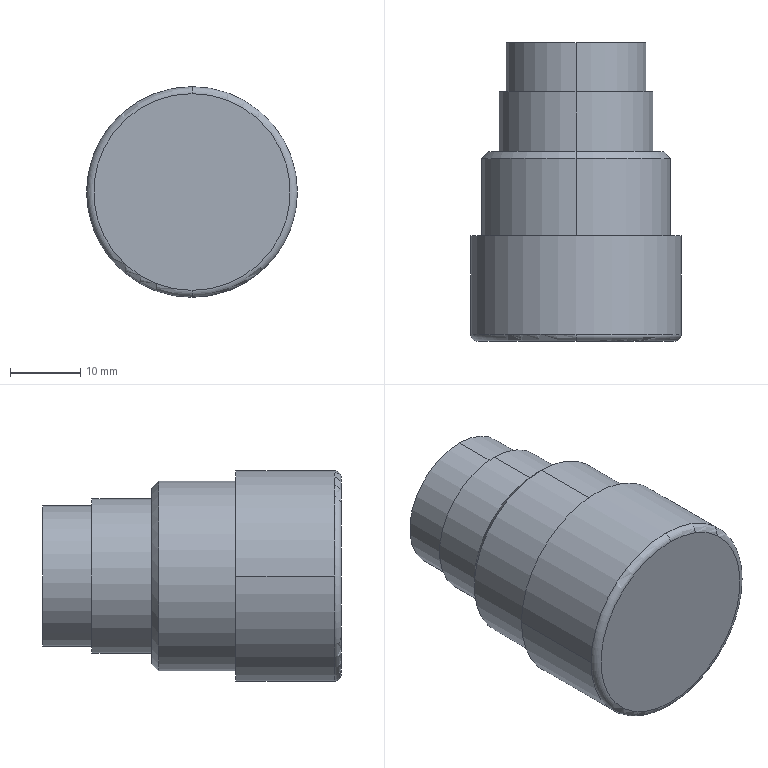Part | SolidWorks | features ICE 2, BaseBody 1, Fillet 1 | 1 solid | 20 faces | box 30 x 42.5 x 30 mm | volume 22079 mm3 | cylinder 10 | plane 6 | torus 2 | cone 2 | commonest cylinder face diameters 18 x2 20 x2 22 x2 27 x2 30 x2
STEP:
#1=CARTESIAN_POINT('',(0.,4.,-14.));
#2=VERTEX_POINT('',#1);
#3=CARTESIAN_POINT('',(0.,4.,14.));
#4=VERTEX_POINT('',#3);
#5=CARTESIAN_POINT('',(0.,4.,0.));
#6=DIRECTION('',(0.,-1.,0.));
#7=DIRECTION('',(0.,0.,1.));
#8=AXIS2_PLACEMENT_3D('',#5,#6,#7);
#9=CIRCLE('',#8,14.);
#10=EDGE_CURVE('',#2,#4,#9,.T.);
#11=ORIENTED_EDGE('',*,*,#10,.F.);
#12=CARTESIAN_POINT('',(0.,5.,-15.));
#13=VERTEX_POINT('',#12);
#14=CARTESIAN_POINT('',(0.,5.,-14.));
#15=DIRECTION('',(1.,0.,0.));
#16=DIRECTION('',(0.,0.,-1.));
#17=AXIS2_PLACEMENT_3D('',#14,#15,#16);
#18=CIRCLE('',#17,1.);
#19=EDGE_CURVE('',#2,#13,#18,.T.);
#20=ORIENTED_EDGE('',*,*,#19,.T.);
#21=CARTESIAN_POINT('',(15.,5.,0.));
#22=VERTEX_POINT('',#21);
#23=CARTESIAN_POINT('',(0.,5.,0.));
#24=DIRECTION('',(0.,1.,0.));
#25=DIRECTION('',(0.,0.,1.));
#26=AXIS2_PLACEMENT_3D('',#23,#24,#25);
#27=CIRCLE('',#26,15.);
#28=EDGE_CURVE('',#22,#13,#27,.T.);
#29=ORIENTED_EDGE('',*,*,#28,.F.);
#30=CARTESIAN_POINT('',(0.,5.,15.));
#31=VERTEX_POINT('',#30);
#32=CARTESIAN_POINT('',(0.,5.,0.));
#33=DIRECTION('',(0.,1.,0.));
#34=DIRECTION('',(0.,0.,1.));
#35=AXIS2_PLACEMENT_3D('',#32,#33,#34);
#36=CIRCLE('',#35,15.);
#37=EDGE_CURVE('',#31,#22,#36,.T.);
#38=ORIENTED_EDGE('',*,*,#37,.F.);
#39=CARTESIAN_POINT('',(0.,5.,14.));
#40=DIRECTION('',(-1.,0.,0.));
#41=DIRECTION('',(0.,0.,1.));
#42=AXIS2_PLACEMENT_3D('',#39,#40,#41);
#43=CIRCLE('',#42,1.);
#44=EDGE_CURVE('',#4,#31,#43,.T.);
#45=ORIENTED_EDGE('',*,*,#44,.F.);
#46=EDGE_LOOP('',(#11,#20,#29,#38,#45));
#47=FACE_OUTER_BOUND('',#46,.T.);
#48=CARTESIAN_POINT('',(0.,5.,0.));
#49=DIRECTION('',(0.,1.,0.));
#50=DIRECTION('',(0.,0.,1.));
#51=AXIS2_PLACEMENT_3D('',#48,#49,#50);
#52=TOROIDAL_SURFACE('',#51,14.,1.);
#53=ADVANCED_FACE('',(#47),#52,.T.);
#54=ORIENTED_EDGE('',*,*,#28,.T.);
#55=CARTESIAN_POINT('',(-15.,5.,0.));
#56=VERTEX_POINT('',#55);
#57=CARTESIAN_POINT('',(0.,5.,0.));
#58=DIRECTION('',(0.,1.,0.));
#59=DIRECTION('',(0.,0.,1.));
#60=AXIS2_PLACEMENT_3D('',#57,#58,#59);
#61=CIRCLE('',#60,15.);
#62=EDGE_CURVE('',#13,#56,#61,.T.);
#63=ORIENTED_EDGE('',*,*,#62,.T.);
#64=CARTESIAN_POINT('',(-15.,19.,0.));
#65=VERTEX_POINT('',#64);
#66=CARTESIAN_POINT('',(-15.,6.,0.));
#67=DIRECTION('',(0.,1.,0.));
#68=VECTOR('',#67,1000.);
#69=LINE('',#66,#68);
#70=EDGE_CURVE('',#56,#65,#69,.T.);
#71=ORIENTED_EDGE('',*,*,#70,.T.);
#72=CARTESIAN_POINT('',(15.,19.,0.));
#73=VERTEX_POINT('',#72);
#74=CARTESIAN_POINT('',(0.,19.,0.));
#75=DIRECTION('',(0.,1.,0.));
#76=DIRECTION('',(1.,0.,0.));
#77=AXIS2_PLACEMENT_3D('',#74,#75,#76);
#78=CIRCLE('',#77,15.);
#79=EDGE_CURVE('',#73,#65,#78,.T.);
#80=ORIENTED_EDGE('',*,*,#79,.F.);
#81=CARTESIAN_POINT('',(15.,6.,0.));
#82=DIRECTION('',(0.,1.,0.));
#83=VECTOR('',#82,1000.);
#84=LINE('',#81,#83);
#85=EDGE_CURVE('',#22,#73,#84,.T.);
#86=ORIENTED_EDGE('',*,*,#85,.F.);
#87=EDGE_LOOP('',(#54,#63,#71,#80,#86));
#88=FACE_OUTER_BOUND('',#87,.T.);
#89=CARTESIAN_POINT('',(0.,6.,0.));
#90=DIRECTION('',(0.,1.,0.));
#91=DIRECTION('',(1.,0.,0.));
#92=AXIS2_PLACEMENT_3D('',#89,#90,#91);
#93=CYLINDRICAL_SURFACE('',#92,15.);
#94=ADVANCED_FACE('',(#88),#93,.T.);
#95=CARTESIAN_POINT('',(9.,43.5,0.));
#96=VERTEX_POINT('',#95);
#97=CARTESIAN_POINT('',(-9.,43.5,0.));
#98=VERTEX_POINT('',#97);
#99=CARTESIAN_POINT('',(0.,43.5,0.));
#100=DIRECTION('',(0.,1.,0.));
#101=DIRECTION('',(1.,0.,0.));
#102=AXIS2_PLACEMENT_3D('',#99,#100,#101);
#103=CIRCLE('',#102,9.);
#104=EDGE_CURVE('',#96,#98,#103,.T.);
#105=ORIENTED_EDGE('',*,*,#104,.T.);
#106=CARTESIAN_POINT('',(0.,43.5,0.));
#107=DIRECTION('',(0.,1.,0.));
#108=DIRECTION('',(-1.,0.,0.));
#109=AXIS2_PLACEMENT_3D('',#106,#107,#108);
#110=CIRCLE('',#109,9.);
#111=EDGE_CURVE('',#98,#96,#110,.T.);
#112=ORIENTED_EDGE('',*,*,#111,.T.);
#113=EDGE_LOOP('',(#105,#112));
#114=FACE_OUTER_BOUND('',#113,.T.);
#115=CARTESIAN_POINT('',(0.,43.5,0.));
#116=DIRECTION('',(0.,1.,0.));
#117=DIRECTION('',(-1.,0.,0.));
#118=AXIS2_PLACEMENT_3D('',#115,#116,#117);
#119=PLANE('',#118);
#120=ADVANCED_FACE('',(#114),#119,.T.);
#121=CARTESIAN_POINT('',(-9.,46.5,0.));
#122=VERTEX_POINT('',#121);
#123=CARTESIAN_POINT('',(-9.,46.5,0.));
#124=DIRECTION('',(0.,-1.,0.));
#125=VECTOR('',#124,1000.);
#126=LINE('',#123,#125);
#127=EDGE_CURVE('',#122,#98,#126,.T.);
#128=ORIENTED_EDGE('',*,*,#127,.T.);
#129=ORIENTED_EDGE('',*,*,#104,.F.);
#130=CARTESIAN_POINT('',(9.,46.5,0.));
#131=VERTEX_POINT('',#130);
#132=CARTESIAN_POINT('',(9.,46.5,0.));
#133=DIRECTION('',(0.,-1.,0.));
#134=VECTOR('',#133,1000.);
#135=LINE('',#132,#134);
#136=EDGE_CURVE('',#131,#96,#135,.T.);
#137=ORIENTED_EDGE('',*,*,#136,.F.);
#138=CARTESIAN_POINT('',(0.,46.5,0.));
#139=DIRECTION('',(0.,1.,0.));
#140=DIRECTION('',(1.,0.,0.));
#141=AXIS2_PLACEMENT_3D('',#138,#139,#140);
#142=CIRCLE('',#141,9.);
#143=EDGE_CURVE('',#131,#122,#142,.T.);
#144=ORIENTED_EDGE('',*,*,#143,.T.);
#145=EDGE_LOOP('',(#128,#129,#137,#144));
#146=FACE_OUTER_BOUND('',#145,.T.);
#147=CARTESIAN_POINT('',(0.,46.5,0.));
#148=DIRECTION('',(0.,1.,0.));
#149=DIRECTION('',(-1.,0.,0.));
#150=AXIS2_PLACEMENT_3D('',#147,#148,#149);
#151=CYLINDRICAL_SURFACE('',#150,9.);
#152=ADVANCED_FACE('',(#146),#151,.F.);
#153=ORIENTED_EDGE('',*,*,#136,.T.);
#154=ORIENTED_EDGE('',*,*,#111,.F.);
#155=ORIENTED_EDGE('',*,*,#127,.F.);
#156=CARTESIAN_POINT('',(0.,46.5,0.));
#157=DIRECTION('',(0.,1.,0.));
#158=DIRECTION('',(-1.,0.,0.));
#159=AXIS2_PLACEMENT_3D('',#156,#157,#158);
#160=CIRCLE('',#159,9.);
#161=EDGE_CURVE('',#122,#131,#160,.T.);
#162=ORIENTED_EDGE('',*,*,#161,.T.);
#163=EDGE_LOOP('',(#153,#154,#155,#162));
#164=FACE_OUTER_BOUND('',#163,.T.);
#165=CARTESIAN_POINT('',(0.,46.5,0.));
#166=DIRECTION('',(0.,1.,0.));
#167=DIRECTION('',(-1.,0.,0.));
#168=AXIS2_PLACEMENT_3D('',#165,#166,#167);
#169=CYLINDRICAL_SURFACE('',#168,9.);
#170=ADVANCED_FACE('',(#164),#169,.F.);
#171=ORIENTED_EDGE('',*,*,#143,.F.);
#172=ORIENTED_EDGE('',*,*,#161,.F.);
#173=EDGE_LOOP('',(#171,#172));
#174=FACE_BOUND('',#173,.T.);
#175=CARTESIAN_POINT('',(0.,46.5,10.));
#176=VERTEX_POINT('',#175);
#177=CARTESIAN_POINT('',(0.,46.5,-10.));
#178=VERTEX_POINT('',#177);
#179=CARTESIAN_POINT('',(0.,46.5,0.));
#180=DIRECTION('',(0.,1.,0.));
#181=DIRECTION('',(0.,0.,1.));
#182=AXIS2_PLACEMENT_3D('',#179,#180,#181);
#183=CIRCLE('',#182,10.);
#184=EDGE_CURVE('',#176,#178,#183,.T.);
#185=ORIENTED_EDGE('',*,*,#184,.T.);
#186=CARTESIAN_POINT('',(0.,46.5,0.));
#187=DIRECTION('',(0.,1.,0.));
#188=DIRECTION('',(0.,0.,-1.));
#189=AXIS2_PLACEMENT_3D('',#186,#187,#188);
#190=CIRCLE('',#189,10.);
#191=EDGE_CURVE('',#178,#176,#190,.T.);
#192=ORIENTED_EDGE('',*,*,#191,.T.);
#193=EDGE_LOOP('',(#185,#192));
#194=FACE_OUTER_BOUND('',#193,.T.);
#195=CARTESIAN_POINT('',(0.,46.5,0.));
#196=DIRECTION('',(0.,1.,0.));
#197=DIRECTION('',(0.,0.,-1.));
#198=AXIS2_PLACEMENT_3D('',#195,#196,#197);
#199=PLANE('',#198);
#200=ADVANCED_FACE('',(#174,#194),#199,.T.);
#201=CARTESIAN_POINT('',(0.,39.5,-10.));
#202=VERTEX_POINT('',#201);
#203=CARTESIAN_POINT('',(0.,39.5,-10.));
#204=DIRECTION('',(0.,1.,0.));
#205=VECTOR('',#204,1000.);
#206=LINE('',#203,#205);
#207=EDGE_CURVE('',#202,#178,#206,.T.);
#208=ORIENTED_EDGE('',*,*,#207,.T.);
#209=ORIENTED_EDGE('',*,*,#184,.F.);
#210=CARTESIAN_POINT('',(0.,39.5,10.));
#211=VERTEX_POINT('',#210);
#212=CARTESIAN_POINT('',(0.,39.5,10.));
#213=DIRECTION('',(0.,1.,0.));
#214=VECTOR('',#213,1000.);
#215=LINE('',#212,#214);
#216=EDGE_CURVE('',#211,#176,#215,.T.);
#217=ORIENTED_EDGE('',*,*,#216,.F.);
#218=CARTESIAN_POINT('',(0.,39.5,0.));
#219=DIRECTION('',(0.,1.,0.));
#220=DIRECTION('',(0.,0.,1.));
#221=AXIS2_PLACEMENT_3D('',#218,#219,#220);
#222=CIRCLE('',#221,10.);
#223=EDGE_CURVE('',#211,#202,#222,.T.);
#224=ORIENTED_EDGE('',*,*,#223,.T.);
#225=EDGE_LOOP('',(#208,#209,#217,#224));
#226=FACE_OUTER_BOUND('',#225,.T.);
#227=CARTESIAN_POINT('',(0.,39.5,0.));
#228=DIRECTION('',(0.,1.,0.));
#229=DIRECTION('',(0.,0.,-1.));
#230=AXIS2_PLACEMENT_3D('',#227,#228,#229);
#231=CYLINDRICAL_SURFACE('',#230,10.);
#232=ADVANCED_FACE('',(#226),#231,.T.);
#233=ORIENTED_EDGE('',*,*,#216,.T.);
#234=ORIENTED_EDGE('',*,*,#191,.F.);
#235=ORIENTED_EDGE('',*,*,#207,.F.);
#236=CARTESIAN_POINT('',(0.,39.5,0.));
#237=DIRECTION('',(0.,1.,0.));
#238=DIRECTION('',(0.,0.,-1.));
#239=AXIS2_PLACEMENT_3D('',#236,#237,#238);
#240=CIRCLE('',#239,10.);
#241=EDGE_CURVE('',#202,#211,#240,.T.);
#242=ORIENTED_EDGE('',*,*,#241,.T.);
#243=EDGE_LOOP('',(#233,#234,#235,#242));
#244=FACE_OUTER_BOUND('',#243,.T.);
#245=CARTESIAN_POINT('',(0.,39.5,0.));
#246=DIRECTION('',(0.,1.,0.));
#247=DIRECTION('',(0.,0.,-1.));
#248=AXIS2_PLACEMENT_3D('',#245,#246,#247);
#249=CYLINDRICAL_SURFACE('',#248,10.);
#250=ADVANCED_FACE('',(#244),#249,.T.);
#251=ORIENTED_EDGE('',*,*,#223,.F.);
#252=ORIENTED_EDGE('',*,*,#241,.F.);
#253=EDGE_LOOP('',(#251,#252));
#254=FACE_BOUND('',#253,.T.);
#255=CARTESIAN_POINT('',(0.,39.5,11.));
#256=VERTEX_POINT('',#255);
#257=CARTESIAN_POINT('',(0.,39.5,-11.));
#258=VERTEX_POINT('',#257);
#259=CARTESIAN_POINT('',(0.,39.5,0.));
#260=DIRECTION('',(0.,1.,0.));
#261=DIRECTION('',(0.,0.,1.));
#262=AXIS2_PLACEMENT_3D('',#259,#260,#261);
#263=CIRCLE('',#262,11.);
#264=EDGE_CURVE('',#256,#258,#263,.T.);
#265=ORIENTED_EDGE('',*,*,#264,.T.);
#266=CARTESIAN_POINT('',(0.,39.5,0.));
#267=DIRECTION('',(0.,1.,0.));
#268=DIRECTION('',(0.,0.,-1.));
#269=AXIS2_PLACEMENT_3D('',#266,#267,#268);
#270=CIRCLE('',#269,11.);
#271=EDGE_CURVE('',#258,#256,#270,.T.);
#272=ORIENTED_EDGE('',*,*,#271,.T.);
#273=EDGE_LOOP('',(#265,#272));
#274=FACE_OUTER_BOUND('',#273,.T.);
#275=CARTESIAN_POINT('',(0.,39.5,0.));
#276=DIRECTION('',(0.,1.,0.));
#277=DIRECTION('',(0.,0.,-1.));
#278=AXIS2_PLACEMENT_3D('',#275,#276,#277);
#279=PLANE('',#278);
#280=ADVANCED_FACE('',(#254,#274),#279,.T.);
#281=CARTESIAN_POINT('',(0.,31.,-11.));
#282=VERTEX_POINT('',#281);
#283=CARTESIAN_POINT('',(0.,31.,-11.));
#284=DIRECTION('',(0.,1.,0.));
#285=VECTOR('',#284,1000.);
#286=LINE('',#283,#285);
#287=EDGE_CURVE('',#282,#258,#286,.T.);
#288=ORIENTED_EDGE('',*,*,#287,.T.);
#289=ORIENTED_EDGE('',*,*,#264,.F.);
#290=CARTESIAN_POINT('',(0.,31.,11.));
#291=VERTEX_POINT('',#290);
#292=CARTESIAN_POINT('',(0.,31.,11.));
#293=DIRECTION('',(0.,1.,0.));
#294=VECTOR('',#293,1000.);
#295=LINE('',#292,#294);
#296=EDGE_CURVE('',#291,#256,#295,.T.);
#297=ORIENTED_EDGE('',*,*,#296,.F.);
#298=CARTESIAN_POINT('',(0.,31.,0.));
#299=DIRECTION('',(0.,1.,0.));
#300=DIRECTION('',(0.,0.,1.));
#301=AXIS2_PLACEMENT_3D('',#298,#299,#300);
#302=CIRCLE('',#301,11.);
#303=EDGE_CURVE('',#291,#282,#302,.T.);
#304=ORIENTED_EDGE('',*,*,#303,.T.);
#305=EDGE_LOOP('',(#288,#289,#297,#304));
#306=FACE_OUTER_BOUND('',#305,.T.);
#307=CARTESIAN_POINT('',(0.,31.,0.));
#308=DIRECTION('',(0.,1.,0.));
#309=DIRECTION('',(0.,0.,-1.));
#310=AXIS2_PLACEMENT_3D('',#307,#308,#309);
#311=CYLINDRICAL_SURFACE('',#310,11.);
#312=ADVANCED_FACE('',(#306),#311,.T.);
#313=ORIENTED_EDGE('',*,*,#296,.T.);
#314=ORIENTED_EDGE('',*,*,#271,.F.);
#315=ORIENTED_EDGE('',*,*,#287,.F.);
#316=CARTESIAN_POINT('',(0.,31.,0.));
#317=DIRECTION('',(0.,1.,0.));
#318=DIRECTION('',(0.,0.,-1.));
#319=AXIS2_PLACEMENT_3D('',#316,#317,#318);
#320=CIRCLE('',#319,11.);
#321=EDGE_CURVE('',#282,#291,#320,.T.);
#322=ORIENTED_EDGE('',*,*,#321,.T.);
#323=EDGE_LOOP('',(#313,#314,#315,#322));
#324=FACE_OUTER_BOUND('',#323,.T.);
#325=CARTESIAN_POINT('',(0.,31.,0.));
#326=DIRECTION('',(0.,1.,0.));
#327=DIRECTION('',(0.,0.,-1.));
#328=AXIS2_PLACEMENT_3D('',#325,#326,#327);
#329=CYLINDRICAL_SURFACE('',#328,11.);
#330=ADVANCED_FACE('',(#324),#329,.T.);
#331=CARTESIAN_POINT('',(0.,19.,13.5));
#332=VERTEX_POINT('',#331);
#333=CARTESIAN_POINT('',(0.000000003,30.,13.5));
#334=VERTEX_POINT('',#333);
#335=CARTESIAN_POINT('',(0.,19.,13.5));
#336=DIRECTION('',(0.,1.,0.));
#337=VECTOR('',#336,1000.);
#338=LINE('',#335,#337);
#339=EDGE_CURVE('',#332,#334,#338,.T.);
#340=ORIENTED_EDGE('',*,*,#339,.F.);
#341=CARTESIAN_POINT('',(0.,19.,-13.5));
#342=VERTEX_POINT('',#341);
#343=CARTESIAN_POINT('',(0.,19.,0.));
#344=DIRECTION('',(0.,1.,0.));
#345=DIRECTION('',(0.,0.,1.));
#346=AXIS2_PLACEMENT_3D('',#343,#344,#345);
#347=CIRCLE('',#346,13.5);
#348=EDGE_CURVE('',#332,#342,#347,.T.);
#349=ORIENTED_EDGE('',*,*,#348,.T.);
#350=CARTESIAN_POINT('',(-0.000000003,30.,-13.5));
#351=VERTEX_POINT('',#350);
#352=CARTESIAN_POINT('',(0.,19.,-13.5));
#353=DIRECTION('',(0.,1.,0.));
#354=VECTOR('',#353,1000.);
#355=LINE('',#352,#354);
#356=EDGE_CURVE('',#342,#351,#355,.T.);
#357=ORIENTED_EDGE('',*,*,#356,.T.);
#358=CARTESIAN_POINT('',(0.,30.,0.));
#359=DIRECTION('',(0.,1.,0.));
#360=DIRECTION('',(0.,0.,1.));
#361=AXIS2_PLACEMENT_3D('',#358,#359,#360);
#362=CIRCLE('',#361,13.5);
#363=EDGE_CURVE('',#334,#351,#362,.T.);
#364=ORIENTED_EDGE('',*,*,#363,.F.);
#365=EDGE_LOOP('',(#340,#349,#357,#364));
#366=FACE_OUTER_BOUND('',#365,.T.);
#367=CARTESIAN_POINT('',(0.,19.,0.));
#368=DIRECTION('',(0.,1.,0.));
#369=DIRECTION('',(0.,0.,-1.));
#370=AXIS2_PLACEMENT_3D('',#367,#368,#369);
#371=CYLINDRICAL_SURFACE('',#370,13.5);
#372=ADVANCED_FACE('',(#366),#371,.T.);
#373=CARTESIAN_POINT('',(0.000000004,31.,12.5));
#374=VERTEX_POINT('',#373);
#375=CARTESIAN_POINT('',(-0.00000005,31.,12.5));
#376=DIRECTION('',(-0.000000003,-0.7071,0.7071));
#377=VECTOR('',#376,1000.);
#378=LINE('',#375,#377);
#379=EDGE_CURVE('',#374,#334,#378,.T.);
#380=ORIENTED_EDGE('',*,*,#379,.T.);
#381=ORIENTED_EDGE('',*,*,#363,.T.);
#382=CARTESIAN_POINT('',(-0.000000004,31.,-12.5));
#383=VERTEX_POINT('',#382);
#384=CARTESIAN_POINT('',(0.00000005,31.,-12.5));
#385=DIRECTION('',(0.000000003,-0.7071,-0.7071));
#386=VECTOR('',#385,1000.);
#387=LINE('',#384,#386);
#388=EDGE_CURVE('',#383,#351,#387,.T.);
#389=ORIENTED_EDGE('',*,*,#388,.F.);
#390=CARTESIAN_POINT('',(0.,31.,0.));
#391=DIRECTION('',(0.,1.,0.));
#392=DIRECTION('',(0.,0.,1.));
#393=AXIS2_PLACEMENT_3D('',#390,#391,#392);
#394=CIRCLE('',#393,12.5);
#395=EDGE_CURVE('',#374,#383,#394,.T.);
#396=ORIENTED_EDGE('',*,*,#395,.F.);
#397=EDGE_LOOP('',(#380,#381,#389,#396));
#398=FACE_OUTER_BOUND('',#397,.T.);
#399=CARTESIAN_POINT('',(0.,31.062,0.));
#400=DIRECTION('',(0.,-1.,0.));
#401=DIRECTION('',(0.,0.,-1.));
#402=AXIS2_PLACEMENT_3D('',#399,#400,#401);
#403=CONICAL_SURFACE('',#402,12.438,0.7854);
#404=ADVANCED_FACE('',(#398),#403,.T.);
#405=ORIENTED_EDGE('',*,*,#303,.F.);
#406=ORIENTED_EDGE('',*,*,#321,.F.);
#407=EDGE_LOOP('',(#405,#406));
#408=FACE_BOUND('',#407,.T.);
#409=CARTESIAN_POINT('',(0.,31.,0.));
#410=DIRECTION('',(0.,1.,0.));
#411=DIRECTION('',(0.,0.,-1.));
#412=AXIS2_PLACEMENT_3D('',#409,#410,#411);
#413=CIRCLE('',#412,12.5);
#414=EDGE_CURVE('',#383,#374,#413,.T.);
#415=ORIENTED_EDGE('',*,*,#414,.T.);
#416=ORIENTED_EDGE('',*,*,#395,.T.);
#417=EDGE_LOOP('',(#415,#416));
#418=FACE_OUTER_BOUND('',#417,.T.);
#419=CARTESIAN_POINT('',(0.,31.,0.));
#420=DIRECTION('',(0.,1.,0.));
#421=DIRECTION('',(0.,0.,-1.));
#422=AXIS2_PLACEMENT_3D('',#419,#420,#421);
#423=PLANE('',#422);
#424=ADVANCED_FACE('',(#408,#418),#423,.T.);
#425=ORIENTED_EDGE('',*,*,#388,.T.);
#426=CARTESIAN_POINT('',(0.,30.,0.));
#427=DIRECTION('',(0.,1.,0.));
#428=DIRECTION('',(0.,0.,-1.));
#429=AXIS2_PLACEMENT_3D('',#426,#427,#428);
#430=CIRCLE('',#429,13.5);
#431=EDGE_CURVE('',#351,#334,#430,.T.);
#432=ORIENTED_EDGE('',*,*,#431,.T.);
#433=ORIENTED_EDGE('',*,*,#379,.F.);
#434=ORIENTED_EDGE('',*,*,#414,.F.);
#435=EDGE_LOOP('',(#425,#432,#433,#434));
#436=FACE_OUTER_BOUND('',#435,.T.);
#437=CARTESIAN_POINT('',(0.,31.062,0.));
#438=DIRECTION('',(0.,-1.,0.));
#439=DIRECTION('',(0.,0.,-1.));
#440=AXIS2_PLACEMENT_3D('',#437,#438,#439);
#441=CONICAL_SURFACE('',#440,12.438,0.7854);
#442=ADVANCED_FACE('',(#436),#441,.T.);
#443=ORIENTED_EDGE('',*,*,#356,.F.);
#444=CARTESIAN_POINT('',(0.,19.,0.));
#445=DIRECTION('',(0.,1.,0.));
#446=DIRECTION('',(0.,0.,-1.));
#447=AXIS2_PLACEMENT_3D('',#444,#445,#446);
#448=CIRCLE('',#447,13.5);
#449=EDGE_CURVE('',#342,#332,#448,.T.);
#450=ORIENTED_EDGE('',*,*,#449,.T.);
#451=ORIENTED_EDGE('',*,*,#339,.T.);
#452=ORIENTED_EDGE('',*,*,#431,.F.);
#453=EDGE_LOOP('',(#443,#450,#451,#452));
#454=FACE_OUTER_BOUND('',#453,.T.);
#455=CARTESIAN_POINT('',(0.,19.,0.));
#456=DIRECTION('',(0.,1.,0.));
#457=DIRECTION('',(0.,0.,-1.));
#458=AXIS2_PLACEMENT_3D('',#455,#456,#457);
#459=CYLINDRICAL_SURFACE('',#458,13.5);
#460=ADVANCED_FACE('',(#454),#459,.T.);
#461=ORIENTED_EDGE('',*,*,#348,.F.);
#462=ORIENTED_EDGE('',*,*,#449,.F.);
#463=EDGE_LOOP('',(#461,#462));
#464=FACE_BOUND('',#463,.T.);
#465=ORIENTED_EDGE('',*,*,#79,.T.);
#466=CARTESIAN_POINT('',(0.,19.,0.));
#467=DIRECTION('',(0.,1.,0.));
#468=DIRECTION('',(1.,0.,0.));
#469=AXIS2_PLACEMENT_3D('',#466,#467,#468);
#470=CIRCLE('',#469,15.);
#471=EDGE_CURVE('',#65,#73,#470,.T.);
#472=ORIENTED_EDGE('',*,*,#471,.T.);
#473=EDGE_LOOP('',(#465,#472));
#474=FACE_OUTER_BOUND('',#473,.T.);
#475=CARTESIAN_POINT('',(0.,19.,0.));
#476=DIRECTION('',(0.,1.,0.));
#477=DIRECTION('',(1.,0.,0.));
#478=AXIS2_PLACEMENT_3D('',#475,#476,#477);
#479=PLANE('',#478);
#480=ADVANCED_FACE('',(#464,#474),#479,.T.);
#481=ORIENTED_EDGE('',*,*,#70,.F.);
#482=CARTESIAN_POINT('',(0.,5.,0.));
#483=DIRECTION('',(0.,1.,0.));
#484=DIRECTION('',(0.,0.,1.));
#485=AXIS2_PLACEMENT_3D('',#482,#483,#484);
#486=CIRCLE('',#485,15.);
#487=EDGE_CURVE('',#56,#31,#486,.T.);
#488=ORIENTED_EDGE('',*,*,#487,.T.);
#489=ORIENTED_EDGE('',*,*,#37,.T.);
#490=ORIENTED_EDGE('',*,*,#85,.T.);
#491=ORIENTED_EDGE('',*,*,#471,.F.);
#492=EDGE_LOOP('',(#481,#488,#489,#490,#491));
#493=FACE_OUTER_BOUND('',#492,.T.);
#494=CARTESIAN_POINT('',(0.,6.,0.));
#495=DIRECTION('',(0.,1.,0.));
#496=DIRECTION('',(1.,0.,0.));
#497=AXIS2_PLACEMENT_3D('',#494,#495,#496);
#498=CYLINDRICAL_SURFACE('',#497,15.);
#499=ADVANCED_FACE('',(#493),#498,.T.);
#500=CARTESIAN_POINT('',(0.,4.,0.));
#501=DIRECTION('',(0.,-1.,0.));
#502=DIRECTION('',(0.,0.,1.));
#503=AXIS2_PLACEMENT_3D('',#500,#501,#502);
#504=CIRCLE('',#503,14.);
#505=EDGE_CURVE('',#4,#2,#504,.T.);
#506=ORIENTED_EDGE('',*,*,#505,.T.);
#507=ORIENTED_EDGE('',*,*,#10,.T.);
#508=EDGE_LOOP('',(#506,#507));
#509=FACE_OUTER_BOUND('',#508,.T.);
#510=CARTESIAN_POINT('',(0.,4.,0.));
#511=DIRECTION('',(0.,1.,0.));
#512=DIRECTION('',(0.,0.,1.));
#513=AXIS2_PLACEMENT_3D('',#510,#511,#512);
#514=PLANE('',#513);
#515=ADVANCED_FACE('',(#509),#514,.F.);
#516=ORIENTED_EDGE('',*,*,#19,.F.);
#517=ORIENTED_EDGE('',*,*,#505,.F.);
#518=ORIENTED_EDGE('',*,*,#44,.T.);
#519=ORIENTED_EDGE('',*,*,#487,.F.);
#520=ORIENTED_EDGE('',*,*,#62,.F.);
#521=EDGE_LOOP('',(#516,#517,#518,#519,#520));
#522=FACE_OUTER_BOUND('',#521,.T.);
#523=CARTESIAN_POINT('',(0.,5.,0.));
#524=DIRECTION('',(0.,1.,0.));
#525=DIRECTION('',(0.,0.,1.));
#526=AXIS2_PLACEMENT_3D('',#523,#524,#525);
#527=TOROIDAL_SURFACE('',#526,14.,1.);
#528=ADVANCED_FACE('',(#522),#527,.T.);
#529=CLOSED_SHELL('',(#53,#94,#120,#152,#170,#200,#232,#250,#280,#312,#330,#372,#404,#424,#442,#460,#480,#499,#515,#528));
#530=MANIFOLD_SOLID_BREP('',#529);
#531=CARTESIAN_POINT('',(0.,0.,0.));
#532=DIRECTION('',(0.,0.,1.));
#533=DIRECTION('',(1.,0.,0.));
#534=AXIS2_PLACEMENT_3D('',#531,#532,#533);
#535=(LENGTH_UNIT()NAMED_UNIT(*)SI_UNIT(.MILLI.,.METRE.));
#536=UNCERTAINTY_MEASURE_WITH_UNIT(LENGTH_MEASURE(0.00001),#535,'','');
#537=(NAMED_UNIT(*)PLANE_ANGLE_UNIT()SI_UNIT($,.RADIAN.));
#538=(NAMED_UNIT(*)SI_UNIT($,.STERADIAN.)SOLID_ANGLE_UNIT());
#539=(GEOMETRIC_REPRESENTATION_CONTEXT(3)GLOBAL_UNCERTAINTY_ASSIGNED_CONTEXT((#536))GLOBAL_UNIT_ASSIGNED_CONTEXT((#535,#537,#538))REPRESENTATION_CONTEXT('',''));
#540=ADVANCED_BREP_SHAPE_REPRESENTATION('',(#530,#534),#539);